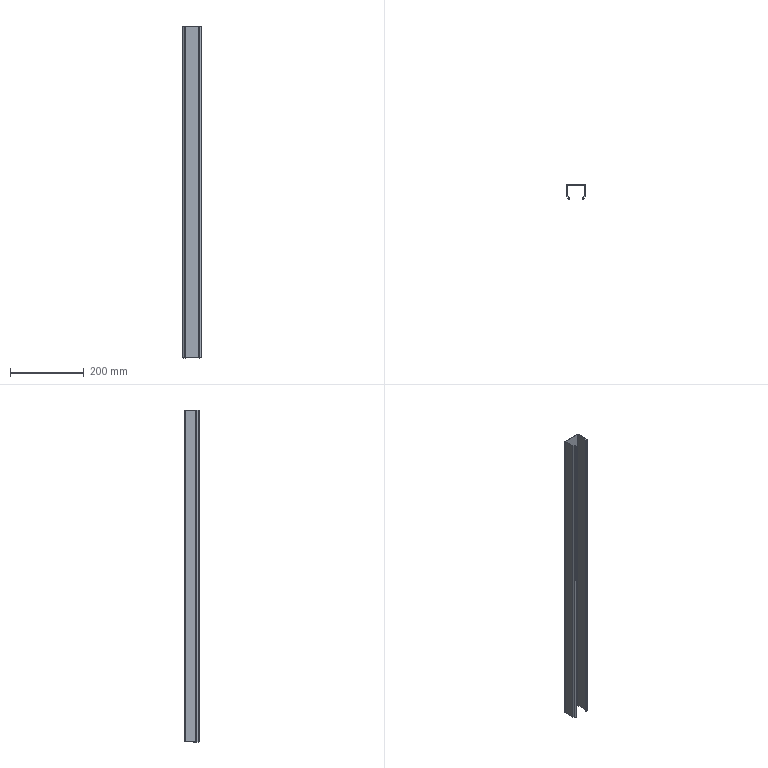Part | STEP file | 31E-01000CC13 | 1 solid | 28 faces | box 50 x 38.192 x 900 mm | volume 148176 mm3 | plane 16 | cylinder 12 | commonest cylinder face diameters 1 x4 2 x4 4 x2 26 x2
STEP:
#1=CARTESIAN_POINT('',(27.993,8.298,900.));
#2=VERTEX_POINT('',#1);
#3=CARTESIAN_POINT('',(32.281,3.187,900.));
#4=VERTEX_POINT('',#3);
#5=CARTESIAN_POINT('',(30.137,5.743,900.));
#6=DIRECTION('',(0.6428,-0.766,0.));
#7=VECTOR('',#6,1.);
#8=LINE('',#5,#7);
#9=EDGE_CURVE('',#2,#4,#8,.T.);
#10=ORIENTED_EDGE('',*,*,#9,.F.);
#11=CARTESIAN_POINT('',(27.993,8.298,0.));
#12=VERTEX_POINT('',#11);
#13=CARTESIAN_POINT('',(27.993,8.298,450.));
#14=DIRECTION('',(0.,0.,-1.));
#15=VECTOR('',#14,1.);
#16=LINE('',#13,#15);
#17=EDGE_CURVE('',#2,#12,#16,.T.);
#18=ORIENTED_EDGE('',*,*,#17,.T.);
#19=CARTESIAN_POINT('',(32.281,3.187,0.));
#20=VERTEX_POINT('',#19);
#21=CARTESIAN_POINT('',(30.137,5.743,0.));
#22=DIRECTION('',(0.6428,-0.766,0.));
#23=VECTOR('',#22,1.);
#24=LINE('',#21,#23);
#25=EDGE_CURVE('',#12,#20,#24,.T.);
#26=ORIENTED_EDGE('',*,*,#25,.T.);
#27=CARTESIAN_POINT('',(32.281,3.187,450.));
#28=DIRECTION('',(0.,0.,-1.));
#29=VECTOR('',#28,1.);
#30=LINE('',#27,#29);
#31=EDGE_CURVE('',#4,#20,#30,.T.);
#32=ORIENTED_EDGE('',*,*,#31,.F.);
#33=EDGE_LOOP('',(#10,#18,#26,#32));
#34=FACE_OUTER_BOUND('',#33,.T.);
#35=CARTESIAN_POINT('',(27.525,8.856,900.));
#36=DIRECTION('',(0.766,0.6428,0.));
#37=DIRECTION('',(-0.6428,0.766,0.));
#38=AXIS2_PLACEMENT_3D('',#35,#36,#37);
#39=PLANE('',#38);
#40=ADVANCED_FACE('',(#34),#39,.F.);
#41=CARTESIAN_POINT('',(76.325,9.293,900.));
#42=VERTEX_POINT('',#41);
#43=CARTESIAN_POINT('',(71.299,3.304,900.));
#44=VERTEX_POINT('',#43);
#45=CARTESIAN_POINT('',(73.812,6.298,900.));
#46=DIRECTION('',(-0.6428,-0.766,0.));
#47=VECTOR('',#46,1.);
#48=LINE('',#45,#47);
#49=EDGE_CURVE('',#42,#44,#48,.T.);
#50=ORIENTED_EDGE('',*,*,#49,.T.);
#51=CARTESIAN_POINT('',(71.182,2.983,900.));
#52=VERTEX_POINT('',#51);
#53=CARTESIAN_POINT('',(71.682,2.983,900.));
#54=DIRECTION('',(0.,0.,1.));
#55=AXIS2_PLACEMENT_3D('',#53,#54,$);
#56=CIRCLE('',#55,0.5);
#57=EDGE_CURVE('',#44,#52,#56,.T.);
#58=ORIENTED_EDGE('',*,*,#57,.T.);
#59=CARTESIAN_POINT('',(71.182,1.665,900.));
#60=VERTEX_POINT('',#59);
#61=CARTESIAN_POINT('',(71.182,2.324,900.));
#62=DIRECTION('',(0.,-1.,0.));
#63=VECTOR('',#62,1.);
#64=LINE('',#61,#63);
#65=EDGE_CURVE('',#52,#60,#64,.T.);
#66=ORIENTED_EDGE('',*,*,#65,.T.);
#67=CARTESIAN_POINT('',(72.397,0.6877,900.));
#68=VERTEX_POINT('',#67);
#69=CARTESIAN_POINT('',(72.182,1.665,900.));
#70=DIRECTION('',(0.,0.,1.));
#71=AXIS2_PLACEMENT_3D('',#69,#70,$);
#72=CIRCLE('',#71,1.);
#73=EDGE_CURVE('',#60,#68,#72,.T.);
#74=ORIENTED_EDGE('',*,*,#73,.T.);
#75=CARTESIAN_POINT('',(76.707,2.493,900.));
#76=VERTEX_POINT('',#75);
#77=CARTESIAN_POINT('',(69.613,13.386,900.));
#78=DIRECTION('',(0.,0.,1.));
#79=AXIS2_PLACEMENT_3D('',#77,#78,$);
#80=CIRCLE('',#79,13.);
#81=EDGE_CURVE('',#68,#76,#80,.T.);
#82=ORIENTED_EDGE('',*,*,#81,.T.);
#83=CARTESIAN_POINT('',(72.768,3.187,900.));
#84=VERTEX_POINT('',#83);
#85=CARTESIAN_POINT('',(74.738,2.84,900.));
#86=DIRECTION('',(-0.9848,0.1736,0.));
#87=VECTOR('',#86,1.);
#88=LINE('',#85,#87);
#89=EDGE_CURVE('',#76,#84,#88,.T.);
#90=ORIENTED_EDGE('',*,*,#89,.T.);
#91=CARTESIAN_POINT('',(77.057,8.298,900.));
#92=VERTEX_POINT('',#91);
#93=CARTESIAN_POINT('',(74.912,5.743,900.));
#94=DIRECTION('',(0.6428,0.766,0.));
#95=VECTOR('',#94,1.);
#96=LINE('',#93,#95);
#97=EDGE_CURVE('',#84,#92,#96,.T.);
#98=ORIENTED_EDGE('',*,*,#97,.T.);
#99=CARTESIAN_POINT('',(77.525,9.584,900.));
#100=VERTEX_POINT('',#99);
#101=CARTESIAN_POINT('',(75.525,9.584,900.));
#102=DIRECTION('',(0.,0.,1.));
#103=AXIS2_PLACEMENT_3D('',#101,#102,$);
#104=CIRCLE('',#103,2.);
#105=EDGE_CURVE('',#92,#100,#104,.T.);
#106=ORIENTED_EDGE('',*,*,#105,.T.);
#107=CARTESIAN_POINT('',(77.525,37.856,900.));
#108=VERTEX_POINT('',#107);
#109=CARTESIAN_POINT('',(77.525,23.72,900.));
#110=DIRECTION('',(0.,1.,0.));
#111=VECTOR('',#110,1.);
#112=LINE('',#109,#111);
#113=EDGE_CURVE('',#100,#108,#112,.T.);
#114=ORIENTED_EDGE('',*,*,#113,.T.);
#115=CARTESIAN_POINT('',(76.525,38.856,900.));
#116=VERTEX_POINT('',#115);
#117=CARTESIAN_POINT('',(76.525,37.856,900.));
#118=DIRECTION('',(0.,0.,1.));
#119=AXIS2_PLACEMENT_3D('',#117,#118,$);
#120=CIRCLE('',#119,1.);
#121=EDGE_CURVE('',#108,#116,#120,.T.);
#122=ORIENTED_EDGE('',*,*,#121,.T.);
#123=CARTESIAN_POINT('',(28.525,38.856,900.));
#124=VERTEX_POINT('',#123);
#125=CARTESIAN_POINT('',(52.525,38.856,900.));
#126=DIRECTION('',(-1.,0.,0.));
#127=VECTOR('',#126,1.);
#128=LINE('',#125,#127);
#129=EDGE_CURVE('',#116,#124,#128,.T.);
#130=ORIENTED_EDGE('',*,*,#129,.T.);
#131=CARTESIAN_POINT('',(27.525,37.856,900.));
#132=VERTEX_POINT('',#131);
#133=CARTESIAN_POINT('',(28.525,37.856,900.));
#134=DIRECTION('',(0.,0.,1.));
#135=AXIS2_PLACEMENT_3D('',#133,#134,$);
#136=CIRCLE('',#135,1.);
#137=EDGE_CURVE('',#124,#132,#136,.T.);
#138=ORIENTED_EDGE('',*,*,#137,.T.);
#139=CARTESIAN_POINT('',(27.525,9.584,900.));
#140=VERTEX_POINT('',#139);
#141=CARTESIAN_POINT('',(27.525,23.72,900.));
#142=DIRECTION('',(0.,-1.,0.));
#143=VECTOR('',#142,1.);
#144=LINE('',#141,#143);
#145=EDGE_CURVE('',#132,#140,#144,.T.);
#146=ORIENTED_EDGE('',*,*,#145,.T.);
#147=CARTESIAN_POINT('',(29.525,9.584,900.));
#148=DIRECTION('',(0.,0.,1.));
#149=AXIS2_PLACEMENT_3D('',#147,#148,$);
#150=CIRCLE('',#149,2.);
#151=EDGE_CURVE('',#140,#2,#150,.T.);
#152=ORIENTED_EDGE('',*,*,#151,.T.);
#153=ORIENTED_EDGE('',*,*,#9,.T.);
#154=CARTESIAN_POINT('',(28.342,2.493,900.));
#155=VERTEX_POINT('',#154);
#156=CARTESIAN_POINT('',(30.312,2.84,900.));
#157=DIRECTION('',(-0.9848,-0.1736,0.));
#158=VECTOR('',#157,1.);
#159=LINE('',#156,#158);
#160=EDGE_CURVE('',#4,#155,#159,.T.);
#161=ORIENTED_EDGE('',*,*,#160,.T.);
#162=CARTESIAN_POINT('',(32.653,0.6877,900.));
#163=VERTEX_POINT('',#162);
#164=CARTESIAN_POINT('',(35.437,13.386,900.));
#165=DIRECTION('',(0.,0.,1.));
#166=AXIS2_PLACEMENT_3D('',#164,#165,$);
#167=CIRCLE('',#166,13.);
#168=EDGE_CURVE('',#155,#163,#167,.T.);
#169=ORIENTED_EDGE('',*,*,#168,.T.);
#170=CARTESIAN_POINT('',(33.867,1.665,900.));
#171=VERTEX_POINT('',#170);
#172=CARTESIAN_POINT('',(32.867,1.665,900.));
#173=DIRECTION('',(0.,0.,1.));
#174=AXIS2_PLACEMENT_3D('',#172,#173,$);
#175=CIRCLE('',#174,1.);
#176=EDGE_CURVE('',#163,#171,#175,.T.);
#177=ORIENTED_EDGE('',*,*,#176,.T.);
#178=CARTESIAN_POINT('',(33.867,2.983,900.));
#179=VERTEX_POINT('',#178);
#180=CARTESIAN_POINT('',(33.867,2.324,900.));
#181=DIRECTION('',(0.,1.,0.));
#182=VECTOR('',#181,1.);
#183=LINE('',#180,#182);
#184=EDGE_CURVE('',#171,#179,#183,.T.);
#185=ORIENTED_EDGE('',*,*,#184,.T.);
#186=CARTESIAN_POINT('',(33.75,3.304,900.));
#187=VERTEX_POINT('',#186);
#188=CARTESIAN_POINT('',(33.367,2.983,900.));
#189=DIRECTION('',(0.,0.,1.));
#190=AXIS2_PLACEMENT_3D('',#188,#189,$);
#191=CIRCLE('',#190,0.5);
#192=EDGE_CURVE('',#179,#187,#191,.T.);
#193=ORIENTED_EDGE('',*,*,#192,.T.);
#194=CARTESIAN_POINT('',(28.725,9.293,900.));
#195=VERTEX_POINT('',#194);
#196=CARTESIAN_POINT('',(31.237,6.298,900.));
#197=DIRECTION('',(-0.6428,0.766,0.));
#198=VECTOR('',#197,1.);
#199=LINE('',#196,#198);
#200=EDGE_CURVE('',#187,#195,#199,.T.);
#201=ORIENTED_EDGE('',*,*,#200,.T.);
#202=CARTESIAN_POINT('',(28.725,37.156,900.));
#203=VERTEX_POINT('',#202);
#204=CARTESIAN_POINT('',(28.725,23.225,900.));
#205=DIRECTION('',(0.,1.,0.));
#206=VECTOR('',#205,1.);
#207=LINE('',#204,#206);
#208=EDGE_CURVE('',#195,#203,#207,.T.);
#209=ORIENTED_EDGE('',*,*,#208,.T.);
#210=CARTESIAN_POINT('',(29.225,37.656,900.));
#211=VERTEX_POINT('',#210);
#212=CARTESIAN_POINT('',(28.725,37.156,900.));
#213=CARTESIAN_POINT('',(28.725,37.219,900.));
#214=CARTESIAN_POINT('',(28.735,37.282,900.));
#215=CARTESIAN_POINT('',(28.754,37.343,900.));
#216=CARTESIAN_POINT('',(28.812,37.456,900.));
#217=CARTESIAN_POINT('',(28.902,37.546,900.));
#218=CARTESIAN_POINT('',(28.954,37.583,900.));
#219=CARTESIAN_POINT('',(29.039,37.627,900.));
#220=CARTESIAN_POINT('',(29.131,37.649,900.));
#221=CARTESIAN_POINT('',(29.162,37.654,900.));
#222=CARTESIAN_POINT('',(29.193,37.656,900.));
#223=CARTESIAN_POINT('',(29.225,37.656,900.));
#224=B_SPLINE_CURVE_WITH_KNOTS('',5,(#212,#213,#214,#215,#216,#217,#218,#219,#220,#221,#222,#223),.UNSPECIFIED.,.F.,.U.,(6,3,3,6),(0.,0.4443,0.8886,1.11),.UNSPECIFIED.);
#225=EDGE_CURVE('',#203,#211,#224,.T.);
#226=ORIENTED_EDGE('',*,*,#225,.T.);
#227=CARTESIAN_POINT('',(75.825,37.656,900.));
#228=VERTEX_POINT('',#227);
#229=CARTESIAN_POINT('',(52.525,37.656,900.));
#230=DIRECTION('',(1.,0.,0.));
#231=VECTOR('',#230,1.);
#232=LINE('',#229,#231);
#233=EDGE_CURVE('',#211,#228,#232,.T.);
#234=ORIENTED_EDGE('',*,*,#233,.T.);
#235=CARTESIAN_POINT('',(76.325,37.156,900.));
#236=VERTEX_POINT('',#235);
#237=CARTESIAN_POINT('',(75.825,37.656,900.));
#238=CARTESIAN_POINT('',(75.888,37.656,900.));
#239=CARTESIAN_POINT('',(75.95,37.646,900.));
#240=CARTESIAN_POINT('',(76.011,37.627,900.));
#241=CARTESIAN_POINT('',(76.124,37.569,900.));
#242=CARTESIAN_POINT('',(76.214,37.479,900.));
#243=CARTESIAN_POINT('',(76.252,37.427,900.));
#244=CARTESIAN_POINT('',(76.295,37.342,900.));
#245=CARTESIAN_POINT('',(76.317,37.25,900.));
#246=CARTESIAN_POINT('',(76.322,37.219,900.));
#247=CARTESIAN_POINT('',(76.325,37.187,900.));
#248=CARTESIAN_POINT('',(76.325,37.156,900.));
#249=B_SPLINE_CURVE_WITH_KNOTS('',5,(#237,#238,#239,#240,#241,#242,#243,#244,#245,#246,#247,#248),.UNSPECIFIED.,.F.,.U.,(6,3,3,6),(0.,0.4443,0.8886,1.11),.UNSPECIFIED.);
#250=EDGE_CURVE('',#228,#236,#249,.T.);
#251=ORIENTED_EDGE('',*,*,#250,.T.);
#252=CARTESIAN_POINT('',(76.325,23.225,900.));
#253=DIRECTION('',(0.,-1.,0.));
#254=VECTOR('',#253,1.);
#255=LINE('',#252,#254);
#256=EDGE_CURVE('',#236,#42,#255,.T.);
#257=ORIENTED_EDGE('',*,*,#256,.T.);
#258=EDGE_LOOP('',(#50,#58,#66,#74,#82,#90,#98,#106,#114,#122,#130,#138,#146,#152,#153,#161,#169,#177,#185,#193,#201,#209,#226,#234,#251,#257));
#259=FACE_OUTER_BOUND('',#258,.T.);
#260=CARTESIAN_POINT('',(35.437,13.386,900.));
#261=DIRECTION('',(0.,0.,1.));
#262=DIRECTION('',(1.,0.,0.));
#263=AXIS2_PLACEMENT_3D('',#260,#261,#262);
#264=PLANE('',#263);
#265=ADVANCED_FACE('',(#259),#264,.T.);
#266=ORIENTED_EDGE('',*,*,#151,.F.);
#267=CARTESIAN_POINT('',(27.525,9.584,0.));
#268=VERTEX_POINT('',#267);
#269=CARTESIAN_POINT('',(27.525,9.584,900.));
#270=DIRECTION('',(0.,0.,-1.));
#271=VECTOR('',#270,1.);
#272=LINE('',#269,#271);
#273=EDGE_CURVE('',#268,#140,#272,.F.);
#274=ORIENTED_EDGE('',*,*,#273,.F.);
#275=CARTESIAN_POINT('',(29.525,9.584,0.));
#276=DIRECTION('',(0.,0.,-1.));
#277=AXIS2_PLACEMENT_3D('',#275,#276,$);
#278=CIRCLE('',#277,2.);
#279=EDGE_CURVE('',#12,#268,#278,.T.);
#280=ORIENTED_EDGE('',*,*,#279,.F.);
#281=ORIENTED_EDGE('',*,*,#17,.F.);
#282=EDGE_LOOP('',(#266,#274,#280,#281));
#283=FACE_OUTER_BOUND('',#282,.T.);
#284=CARTESIAN_POINT('',(29.525,9.584,900.));
#285=DIRECTION('',(0.,0.,-1.));
#286=DIRECTION('',(1.,0.,0.));
#287=AXIS2_PLACEMENT_3D('',#284,#285,#286);
#288=CYLINDRICAL_SURFACE('',#287,2.);
#289=ADVANCED_FACE('',(#283),#288,.T.);
#290=CARTESIAN_POINT('',(71.182,2.983,0.));
#291=VERTEX_POINT('',#290);
#292=CARTESIAN_POINT('',(71.182,1.665,0.));
#293=VERTEX_POINT('',#292);
#294=CARTESIAN_POINT('',(71.182,2.324,0.));
#295=DIRECTION('',(0.,-1.,0.));
#296=VECTOR('',#295,1.);
#297=LINE('',#294,#296);
#298=EDGE_CURVE('',#291,#293,#297,.T.);
#299=ORIENTED_EDGE('',*,*,#298,.F.);
#300=CARTESIAN_POINT('',(71.299,3.304,0.));
#301=VERTEX_POINT('',#300);
#302=CARTESIAN_POINT('',(71.182,2.983,0.));
#303=CARTESIAN_POINT('',(71.182,3.038,0.));
#304=CARTESIAN_POINT('',(71.19,3.094,0.));
#305=CARTESIAN_POINT('',(71.206,3.149,0.));
#306=CARTESIAN_POINT('',(71.235,3.213,0.));
#307=CARTESIAN_POINT('',(71.274,3.271,0.));
#308=CARTESIAN_POINT('',(71.282,3.282,0.));
#309=CARTESIAN_POINT('',(71.29,3.293,0.));
#310=CARTESIAN_POINT('',(71.299,3.304,0.));
#311=B_SPLINE_CURVE_WITH_KNOTS('',5,(#302,#303,#304,#305,#306,#307,#308,#309,#310),.UNSPECIFIED.,.F.,.U.,(6,3,6),(0.,0.3949,0.4936),.UNSPECIFIED.);
#312=EDGE_CURVE('',#291,#301,#311,.T.);
#313=ORIENTED_EDGE('',*,*,#312,.T.);
#314=CARTESIAN_POINT('',(76.325,9.293,0.));
#315=VERTEX_POINT('',#314);
#316=CARTESIAN_POINT('',(73.812,6.298,0.));
#317=DIRECTION('',(-0.6428,-0.766,0.));
#318=VECTOR('',#317,1.);
#319=LINE('',#316,#318);
#320=EDGE_CURVE('',#315,#301,#319,.T.);
#321=ORIENTED_EDGE('',*,*,#320,.F.);
#322=CARTESIAN_POINT('',(76.325,37.156,0.));
#323=VERTEX_POINT('',#322);
#324=CARTESIAN_POINT('',(76.325,23.225,0.));
#325=DIRECTION('',(0.,-1.,0.));
#326=VECTOR('',#325,1.);
#327=LINE('',#324,#326);
#328=EDGE_CURVE('',#323,#315,#327,.T.);
#329=ORIENTED_EDGE('',*,*,#328,.F.);
#330=CARTESIAN_POINT('',(75.825,37.656,0.));
#331=VERTEX_POINT('',#330);
#332=CARTESIAN_POINT('',(75.825,37.156,0.));
#333=DIRECTION('',(0.,0.,1.));
#334=AXIS2_PLACEMENT_3D('',#332,#333,$);
#335=CIRCLE('',#334,0.5);
#336=EDGE_CURVE('',#323,#331,#335,.T.);
#337=ORIENTED_EDGE('',*,*,#336,.T.);
#338=CARTESIAN_POINT('',(29.225,37.656,0.));
#339=VERTEX_POINT('',#338);
#340=CARTESIAN_POINT('',(52.525,37.656,0.));
#341=DIRECTION('',(1.,0.,0.));
#342=VECTOR('',#341,1.);
#343=LINE('',#340,#342);
#344=EDGE_CURVE('',#339,#331,#343,.T.);
#345=ORIENTED_EDGE('',*,*,#344,.F.);
#346=CARTESIAN_POINT('',(28.725,37.156,0.));
#347=VERTEX_POINT('',#346);
#348=CARTESIAN_POINT('',(29.225,37.156,0.));
#349=DIRECTION('',(0.,0.,1.));
#350=AXIS2_PLACEMENT_3D('',#348,#349,$);
#351=CIRCLE('',#350,0.5);
#352=EDGE_CURVE('',#339,#347,#351,.T.);
#353=ORIENTED_EDGE('',*,*,#352,.T.);
#354=CARTESIAN_POINT('',(28.725,9.293,0.));
#355=VERTEX_POINT('',#354);
#356=CARTESIAN_POINT('',(28.725,23.225,0.));
#357=DIRECTION('',(0.,1.,0.));
#358=VECTOR('',#357,1.);
#359=LINE('',#356,#358);
#360=EDGE_CURVE('',#355,#347,#359,.T.);
#361=ORIENTED_EDGE('',*,*,#360,.F.);
#362=CARTESIAN_POINT('',(33.75,3.304,0.));
#363=VERTEX_POINT('',#362);
#364=CARTESIAN_POINT('',(31.237,6.298,0.));
#365=DIRECTION('',(-0.6428,0.766,0.));
#366=VECTOR('',#365,1.);
#367=LINE('',#364,#366);
#368=EDGE_CURVE('',#363,#355,#367,.T.);
#369=ORIENTED_EDGE('',*,*,#368,.F.);
#370=CARTESIAN_POINT('',(33.867,2.983,0.));
#371=VERTEX_POINT('',#370);
#372=CARTESIAN_POINT('',(33.75,3.304,0.));
#373=CARTESIAN_POINT('',(33.786,3.261,0.));
#374=CARTESIAN_POINT('',(33.816,3.213,0.));
#375=CARTESIAN_POINT('',(33.839,3.162,0.));
#376=CARTESIAN_POINT('',(33.858,3.094,0.));
#377=CARTESIAN_POINT('',(33.866,3.024,0.));
#378=CARTESIAN_POINT('',(33.867,3.01,0.));
#379=CARTESIAN_POINT('',(33.867,2.997,0.));
#380=CARTESIAN_POINT('',(33.867,2.983,0.));
#381=B_SPLINE_CURVE_WITH_KNOTS('',5,(#372,#373,#374,#375,#376,#377,#378,#379,#380),.UNSPECIFIED.,.F.,.U.,(6,3,6),(0.,0.3949,0.4936),.UNSPECIFIED.);
#382=EDGE_CURVE('',#363,#371,#381,.T.);
#383=ORIENTED_EDGE('',*,*,#382,.T.);
#384=CARTESIAN_POINT('',(33.867,1.665,0.));
#385=VERTEX_POINT('',#384);
#386=CARTESIAN_POINT('',(33.867,2.324,0.));
#387=DIRECTION('',(0.,1.,0.));
#388=VECTOR('',#387,1.);
#389=LINE('',#386,#388);
#390=EDGE_CURVE('',#385,#371,#389,.T.);
#391=ORIENTED_EDGE('',*,*,#390,.F.);
#392=CARTESIAN_POINT('',(32.653,0.6877,0.));
#393=VERTEX_POINT('',#392);
#394=CARTESIAN_POINT('',(32.867,1.665,0.));
#395=DIRECTION('',(0.,0.,1.));
#396=AXIS2_PLACEMENT_3D('',#394,#395,$);
#397=CIRCLE('',#396,1.);
#398=EDGE_CURVE('',#393,#385,#397,.T.);
#399=ORIENTED_EDGE('',*,*,#398,.F.);
#400=CARTESIAN_POINT('',(28.342,2.493,0.));
#401=VERTEX_POINT('',#400);
#402=CARTESIAN_POINT('',(35.437,13.386,0.));
#403=DIRECTION('',(0.,0.,1.));
#404=AXIS2_PLACEMENT_3D('',#402,#403,$);
#405=CIRCLE('',#404,13.);
#406=EDGE_CURVE('',#401,#393,#405,.T.);
#407=ORIENTED_EDGE('',*,*,#406,.F.);
#408=CARTESIAN_POINT('',(30.312,2.84,0.));
#409=DIRECTION('',(-0.9848,-0.1736,0.));
#410=VECTOR('',#409,1.);
#411=LINE('',#408,#410);
#412=EDGE_CURVE('',#20,#401,#411,.T.);
#413=ORIENTED_EDGE('',*,*,#412,.F.);
#414=ORIENTED_EDGE('',*,*,#25,.F.);
#415=ORIENTED_EDGE('',*,*,#279,.T.);
#416=CARTESIAN_POINT('',(27.525,37.856,0.));
#417=VERTEX_POINT('',#416);
#418=CARTESIAN_POINT('',(27.525,23.72,0.));
#419=DIRECTION('',(0.,-1.,0.));
#420=VECTOR('',#419,1.);
#421=LINE('',#418,#420);
#422=EDGE_CURVE('',#417,#268,#421,.T.);
#423=ORIENTED_EDGE('',*,*,#422,.F.);
#424=CARTESIAN_POINT('',(28.525,38.856,0.));
#425=VERTEX_POINT('',#424);
#426=CARTESIAN_POINT('',(27.525,37.856,0.));
#427=CARTESIAN_POINT('',(27.525,37.954,0.));
#428=CARTESIAN_POINT('',(27.537,38.052,0.));
#429=CARTESIAN_POINT('',(27.561,38.148,0.));
#430=CARTESIAN_POINT('',(27.632,38.332,0.));
#431=CARTESIAN_POINT('',(27.745,38.494,0.));
#432=CARTESIAN_POINT('',(27.812,38.567,0.));
#433=CARTESIAN_POINT('',(27.961,38.696,0.));
#434=CARTESIAN_POINT('',(28.137,38.786,0.));
#435=CARTESIAN_POINT('',(28.23,38.819,0.));
#436=CARTESIAN_POINT('',(28.346,38.846,0.));
#437=CARTESIAN_POINT('',(28.464,38.855,0.));
#438=CARTESIAN_POINT('',(28.484,38.856,0.));
#439=CARTESIAN_POINT('',(28.505,38.856,0.));
#440=CARTESIAN_POINT('',(28.525,38.856,0.));
#441=B_SPLINE_CURVE_WITH_KNOTS('',5,(#426,#427,#428,#429,#430,#431,#432,#433,#434,#435,#436,#437,#438,#439,#440),.UNSPECIFIED.,.F.,.U.,(6,3,3,3,6),(0.,0.6928,1.386,2.078,2.221),.UNSPECIFIED.);
#442=EDGE_CURVE('',#417,#425,#441,.T.);
#443=ORIENTED_EDGE('',*,*,#442,.T.);
#444=CARTESIAN_POINT('',(76.525,38.856,0.));
#445=VERTEX_POINT('',#444);
#446=CARTESIAN_POINT('',(52.525,38.856,0.));
#447=DIRECTION('',(-1.,0.,0.));
#448=VECTOR('',#447,1.);
#449=LINE('',#446,#448);
#450=EDGE_CURVE('',#445,#425,#449,.T.);
#451=ORIENTED_EDGE('',*,*,#450,.F.);
#452=CARTESIAN_POINT('',(77.525,37.856,0.));
#453=VERTEX_POINT('',#452);
#454=CARTESIAN_POINT('',(76.525,38.856,0.));
#455=CARTESIAN_POINT('',(76.623,38.856,0.));
#456=CARTESIAN_POINT('',(76.721,38.844,0.));
#457=CARTESIAN_POINT('',(76.817,38.82,0.));
#458=CARTESIAN_POINT('',(77.001,38.749,0.));
#459=CARTESIAN_POINT('',(77.163,38.636,0.));
#460=CARTESIAN_POINT('',(77.236,38.569,0.));
#461=CARTESIAN_POINT('',(77.365,38.42,0.));
#462=CARTESIAN_POINT('',(77.454,38.244,0.));
#463=CARTESIAN_POINT('',(77.488,38.151,0.));
#464=CARTESIAN_POINT('',(77.514,38.035,0.));
#465=CARTESIAN_POINT('',(77.523,37.917,0.));
#466=CARTESIAN_POINT('',(77.524,37.897,0.));
#467=CARTESIAN_POINT('',(77.525,37.876,0.));
#468=CARTESIAN_POINT('',(77.525,37.856,0.));
#469=B_SPLINE_CURVE_WITH_KNOTS('',5,(#454,#455,#456,#457,#458,#459,#460,#461,#462,#463,#464,#465,#466,#467,#468),.UNSPECIFIED.,.F.,.U.,(6,3,3,3,6),(0.,0.6928,1.386,2.078,2.221),.UNSPECIFIED.);
#470=EDGE_CURVE('',#445,#453,#469,.T.);
#471=ORIENTED_EDGE('',*,*,#470,.T.);
#472=CARTESIAN_POINT('',(77.525,9.584,0.));
#473=VERTEX_POINT('',#472);
#474=CARTESIAN_POINT('',(77.525,23.72,0.));
#475=DIRECTION('',(0.,1.,0.));
#476=VECTOR('',#475,1.);
#477=LINE('',#474,#476);
#478=EDGE_CURVE('',#473,#453,#477,.T.);
#479=ORIENTED_EDGE('',*,*,#478,.F.);
#480=CARTESIAN_POINT('',(77.057,8.298,0.));
#481=VERTEX_POINT('',#480);
#482=CARTESIAN_POINT('',(77.525,9.584,0.));
#483=CARTESIAN_POINT('',(77.525,9.361,0.));
#484=CARTESIAN_POINT('',(77.494,9.137,0.));
#485=CARTESIAN_POINT('',(77.431,8.92,0.));
#486=CARTESIAN_POINT('',(77.316,8.662,0.));
#487=CARTESIAN_POINT('',(77.16,8.431,0.));
#488=CARTESIAN_POINT('',(77.127,8.385,0.));
#489=CARTESIAN_POINT('',(77.093,8.341,0.));
#490=CARTESIAN_POINT('',(77.057,8.298,0.));
#491=B_SPLINE_CURVE_WITH_KNOTS('',5,(#482,#483,#484,#485,#486,#487,#488,#489,#490),.UNSPECIFIED.,.F.,.U.,(6,3,6),(0.,1.58,1.974),.UNSPECIFIED.);
#492=EDGE_CURVE('',#473,#481,#491,.T.);
#493=ORIENTED_EDGE('',*,*,#492,.T.);
#494=CARTESIAN_POINT('',(72.768,3.187,0.));
#495=VERTEX_POINT('',#494);
#496=CARTESIAN_POINT('',(74.912,5.743,0.));
#497=DIRECTION('',(0.6428,0.766,0.));
#498=VECTOR('',#497,1.);
#499=LINE('',#496,#498);
#500=EDGE_CURVE('',#495,#481,#499,.T.);
#501=ORIENTED_EDGE('',*,*,#500,.F.);
#502=CARTESIAN_POINT('',(76.707,2.493,0.));
#503=VERTEX_POINT('',#502);
#504=CARTESIAN_POINT('',(74.738,2.84,0.));
#505=DIRECTION('',(-0.9848,0.1736,0.));
#506=VECTOR('',#505,1.);
#507=LINE('',#504,#506);
#508=EDGE_CURVE('',#503,#495,#507,.T.);
#509=ORIENTED_EDGE('',*,*,#508,.F.);
#510=CARTESIAN_POINT('',(72.397,0.6877,0.));
#511=VERTEX_POINT('',#510);
#512=CARTESIAN_POINT('',(69.613,13.386,0.));
#513=DIRECTION('',(0.,0.,1.));
#514=AXIS2_PLACEMENT_3D('',#512,#513,$);
#515=CIRCLE('',#514,13.);
#516=EDGE_CURVE('',#511,#503,#515,.T.);
#517=ORIENTED_EDGE('',*,*,#516,.F.);
#518=CARTESIAN_POINT('',(72.182,1.665,0.));
#519=DIRECTION('',(0.,0.,1.));
#520=AXIS2_PLACEMENT_3D('',#518,#519,$);
#521=CIRCLE('',#520,1.);
#522=EDGE_CURVE('',#293,#511,#521,.T.);
#523=ORIENTED_EDGE('',*,*,#522,.F.);
#524=EDGE_LOOP('',(#299,#313,#321,#329,#337,#345,#353,#361,#369,#383,#391,#399,#407,#413,#414,#415,#423,#443,#451,#471,#479,#493,#501,#509,#517,#523));
#525=FACE_OUTER_BOUND('',#524,.T.);
#526=CARTESIAN_POINT('',(35.437,13.386,0.));
#527=DIRECTION('',(0.,0.,1.));
#528=DIRECTION('',(1.,0.,0.));
#529=AXIS2_PLACEMENT_3D('',#526,#527,#528);
#530=PLANE('',#529);
#531=ADVANCED_FACE('',(#525),#530,.F.);
#532=ORIENTED_EDGE('',*,*,#412,.T.);
#533=CARTESIAN_POINT('',(28.342,2.493,450.));
#534=DIRECTION('',(0.,0.,-1.));
#535=VECTOR('',#534,1.);
#536=LINE('',#533,#535);
#537=EDGE_CURVE('',#155,#401,#536,.T.);
#538=ORIENTED_EDGE('',*,*,#537,.F.);
#539=ORIENTED_EDGE('',*,*,#160,.F.);
#540=ORIENTED_EDGE('',*,*,#31,.T.);
#541=EDGE_LOOP('',(#532,#538,#539,#540));
#542=FACE_OUTER_BOUND('',#541,.T.);
#543=CARTESIAN_POINT('',(32.281,3.187,900.));
#544=DIRECTION('',(0.1736,-0.9848,0.));
#545=DIRECTION('',(0.9848,0.1736,0.));
#546=AXIS2_PLACEMENT_3D('',#543,#544,#545);
#547=PLANE('',#546);
#548=ADVANCED_FACE('',(#542),#547,.F.);
#549=ORIENTED_EDGE('',*,*,#320,.T.);
#550=CARTESIAN_POINT('',(71.299,3.304,450.));
#551=DIRECTION('',(0.,0.,1.));
#552=VECTOR('',#551,1.);
#553=LINE('',#550,#552);
#554=EDGE_CURVE('',#301,#44,#553,.T.);
#555=ORIENTED_EDGE('',*,*,#554,.T.);
#556=ORIENTED_EDGE('',*,*,#49,.F.);
#557=CARTESIAN_POINT('',(76.325,9.293,450.));
#558=DIRECTION('',(0.,0.,-1.));
#559=VECTOR('',#558,1.);
#560=LINE('',#557,#559);
#561=EDGE_CURVE('',#42,#315,#560,.T.);
#562=ORIENTED_EDGE('',*,*,#561,.T.);
#563=EDGE_LOOP('',(#549,#555,#556,#562));
#564=FACE_OUTER_BOUND('',#563,.T.);
#565=CARTESIAN_POINT('',(76.325,9.293,900.));
#566=DIRECTION('',(0.766,-0.6428,0.));
#567=DIRECTION('',(0.6428,0.766,0.));
#568=AXIS2_PLACEMENT_3D('',#565,#566,#567);
#569=PLANE('',#568);
#570=ADVANCED_FACE('',(#564),#569,.F.);
#571=ORIENTED_EDGE('',*,*,#57,.F.);
#572=ORIENTED_EDGE('',*,*,#554,.F.);
#573=ORIENTED_EDGE('',*,*,#312,.F.);
#574=CARTESIAN_POINT('',(71.182,2.983,900.));
#575=DIRECTION('',(0.,0.,-1.));
#576=VECTOR('',#575,1.);
#577=LINE('',#574,#576);
#578=EDGE_CURVE('',#52,#291,#577,.T.);
#579=ORIENTED_EDGE('',*,*,#578,.F.);
#580=EDGE_LOOP('',(#571,#572,#573,#579));
#581=FACE_OUTER_BOUND('',#580,.T.);
#582=CARTESIAN_POINT('',(71.682,2.983,900.));
#583=DIRECTION('',(0.,0.,-1.));
#584=DIRECTION('',(-1.,0.,0.));
#585=AXIS2_PLACEMENT_3D('',#582,#583,#584);
#586=CYLINDRICAL_SURFACE('',#585,0.5);
#587=ADVANCED_FACE('',(#581),#586,.T.);
#588=ORIENTED_EDGE('',*,*,#65,.F.);
#589=ORIENTED_EDGE('',*,*,#578,.T.);
#590=ORIENTED_EDGE('',*,*,#298,.T.);
#591=CARTESIAN_POINT('',(71.182,1.665,450.));
#592=DIRECTION('',(0.,0.,-1.));
#593=VECTOR('',#592,1.);
#594=LINE('',#591,#593);
#595=EDGE_CURVE('',#60,#293,#594,.T.);
#596=ORIENTED_EDGE('',*,*,#595,.F.);
#597=EDGE_LOOP('',(#588,#589,#590,#596));
#598=FACE_OUTER_BOUND('',#597,.T.);
#599=CARTESIAN_POINT('',(71.182,1.665,900.));
#600=DIRECTION('',(1.,0.,0.));
#601=DIRECTION('',(0.,0.,-1.));
#602=AXIS2_PLACEMENT_3D('',#599,#600,#601);
#603=PLANE('',#602);
#604=ADVANCED_FACE('',(#598),#603,.F.);
#605=ORIENTED_EDGE('',*,*,#522,.T.);
#606=CARTESIAN_POINT('',(72.397,0.6877,900.));
#607=DIRECTION('',(0.,0.,-1.));
#608=VECTOR('',#607,1.);
#609=LINE('',#606,#608);
#610=EDGE_CURVE('',#68,#511,#609,.T.);
#611=ORIENTED_EDGE('',*,*,#610,.F.);
#612=ORIENTED_EDGE('',*,*,#73,.F.);
#613=ORIENTED_EDGE('',*,*,#595,.T.);
#614=EDGE_LOOP('',(#605,#611,#612,#613));
#615=FACE_OUTER_BOUND('',#614,.T.);
#616=CARTESIAN_POINT('',(72.182,1.665,900.));
#617=DIRECTION('',(0.,0.,-1.));
#618=DIRECTION('',(1.,0.,0.));
#619=AXIS2_PLACEMENT_3D('',#616,#617,#618);
#620=CYLINDRICAL_SURFACE('',#619,1.);
#621=ADVANCED_FACE('',(#615),#620,.T.);
#622=ORIENTED_EDGE('',*,*,#516,.T.);
#623=CARTESIAN_POINT('',(76.707,2.493,900.));
#624=DIRECTION('',(0.,0.,-1.));
#625=VECTOR('',#624,1.);
#626=LINE('',#623,#625);
#627=EDGE_CURVE('',#76,#503,#626,.T.);
#628=ORIENTED_EDGE('',*,*,#627,.F.);
#629=ORIENTED_EDGE('',*,*,#81,.F.);
#630=ORIENTED_EDGE('',*,*,#610,.T.);
#631=EDGE_LOOP('',(#622,#628,#629,#630));
#632=FACE_OUTER_BOUND('',#631,.T.);
#633=CARTESIAN_POINT('',(69.613,13.386,900.));
#634=DIRECTION('',(0.,0.,-1.));
#635=DIRECTION('',(1.,0.,0.));
#636=AXIS2_PLACEMENT_3D('',#633,#634,#635);
#637=CYLINDRICAL_SURFACE('',#636,13.);
#638=ADVANCED_FACE('',(#632),#637,.T.);
#639=ORIENTED_EDGE('',*,*,#508,.T.);
#640=CARTESIAN_POINT('',(72.768,3.187,450.));
#641=DIRECTION('',(0.,0.,-1.));
#642=VECTOR('',#641,1.);
#643=LINE('',#640,#642);
#644=EDGE_CURVE('',#84,#495,#643,.T.);
#645=ORIENTED_EDGE('',*,*,#644,.F.);
#646=ORIENTED_EDGE('',*,*,#89,.F.);
#647=ORIENTED_EDGE('',*,*,#627,.T.);
#648=EDGE_LOOP('',(#639,#645,#646,#647));
#649=FACE_OUTER_BOUND('',#648,.T.);
#650=CARTESIAN_POINT('',(72.768,3.187,900.));
#651=DIRECTION('',(-0.1736,-0.9848,0.));
#652=DIRECTION('',(0.9848,-0.1736,0.));
#653=AXIS2_PLACEMENT_3D('',#650,#651,#652);
#654=PLANE('',#653);
#655=ADVANCED_FACE('',(#649),#654,.F.);
#656=ORIENTED_EDGE('',*,*,#500,.T.);
#657=CARTESIAN_POINT('',(77.057,8.298,450.));
#658=DIRECTION('',(0.,0.,1.));
#659=VECTOR('',#658,1.);
#660=LINE('',#657,#659);
#661=EDGE_CURVE('',#481,#92,#660,.T.);
#662=ORIENTED_EDGE('',*,*,#661,.T.);
#663=ORIENTED_EDGE('',*,*,#97,.F.);
#664=ORIENTED_EDGE('',*,*,#644,.T.);
#665=EDGE_LOOP('',(#656,#662,#663,#664));
#666=FACE_OUTER_BOUND('',#665,.T.);
#667=CARTESIAN_POINT('',(77.525,8.856,900.));
#668=DIRECTION('',(-0.766,0.6428,0.));
#669=DIRECTION('',(-0.6428,-0.766,0.));
#670=AXIS2_PLACEMENT_3D('',#667,#668,#669);
#671=PLANE('',#670);
#672=ADVANCED_FACE('',(#666),#671,.F.);
#673=ORIENTED_EDGE('',*,*,#105,.F.);
#674=ORIENTED_EDGE('',*,*,#661,.F.);
#675=ORIENTED_EDGE('',*,*,#492,.F.);
#676=CARTESIAN_POINT('',(77.525,9.584,900.));
#677=DIRECTION('',(0.,0.,-1.));
#678=VECTOR('',#677,1.);
#679=LINE('',#676,#678);
#680=EDGE_CURVE('',#100,#473,#679,.T.);
#681=ORIENTED_EDGE('',*,*,#680,.F.);
#682=EDGE_LOOP('',(#673,#674,#675,#681));
#683=FACE_OUTER_BOUND('',#682,.T.);
#684=CARTESIAN_POINT('',(75.525,9.584,900.));
#685=DIRECTION('',(0.,0.,-1.));
#686=DIRECTION('',(1.,0.,0.));
#687=AXIS2_PLACEMENT_3D('',#684,#685,#686);
#688=CYLINDRICAL_SURFACE('',#687,2.);
#689=ADVANCED_FACE('',(#683),#688,.T.);
#690=ORIENTED_EDGE('',*,*,#478,.T.);
#691=CARTESIAN_POINT('',(77.525,37.856,450.));
#692=DIRECTION('',(0.,0.,1.));
#693=VECTOR('',#692,1.);
#694=LINE('',#691,#693);
#695=EDGE_CURVE('',#453,#108,#694,.T.);
#696=ORIENTED_EDGE('',*,*,#695,.T.);
#697=ORIENTED_EDGE('',*,*,#113,.F.);
#698=ORIENTED_EDGE('',*,*,#680,.T.);
#699=EDGE_LOOP('',(#690,#696,#697,#698));
#700=FACE_OUTER_BOUND('',#699,.T.);
#701=CARTESIAN_POINT('',(77.525,8.856,900.));
#702=DIRECTION('',(-1.,0.,0.));
#703=DIRECTION('',(0.,0.,1.));
#704=AXIS2_PLACEMENT_3D('',#701,#702,#703);
#705=PLANE('',#704);
#706=ADVANCED_FACE('',(#700),#705,.F.);
#707=ORIENTED_EDGE('',*,*,#121,.F.);
#708=ORIENTED_EDGE('',*,*,#695,.F.);
#709=ORIENTED_EDGE('',*,*,#470,.F.);
#710=CARTESIAN_POINT('',(76.525,38.856,900.));
#711=DIRECTION('',(0.,0.,-1.));
#712=VECTOR('',#711,1.);
#713=LINE('',#710,#712);
#714=EDGE_CURVE('',#116,#445,#713,.T.);
#715=ORIENTED_EDGE('',*,*,#714,.F.);
#716=EDGE_LOOP('',(#707,#708,#709,#715));
#717=FACE_OUTER_BOUND('',#716,.T.);
#718=CARTESIAN_POINT('',(76.525,37.856,900.));
#719=DIRECTION('',(0.,0.,-1.));
#720=DIRECTION('',(-1.,0.,0.));
#721=AXIS2_PLACEMENT_3D('',#718,#719,#720);
#722=CYLINDRICAL_SURFACE('',#721,1.);
#723=ADVANCED_FACE('',(#717),#722,.T.);
#724=ORIENTED_EDGE('',*,*,#129,.F.);
#725=ORIENTED_EDGE('',*,*,#714,.T.);
#726=ORIENTED_EDGE('',*,*,#450,.T.);
#727=CARTESIAN_POINT('',(28.525,38.856,450.));
#728=DIRECTION('',(0.,0.,1.));
#729=VECTOR('',#728,1.);
#730=LINE('',#727,#729);
#731=EDGE_CURVE('',#425,#124,#730,.T.);
#732=ORIENTED_EDGE('',*,*,#731,.T.);
#733=EDGE_LOOP('',(#724,#725,#726,#732));
#734=FACE_OUTER_BOUND('',#733,.T.);
#735=CARTESIAN_POINT('',(27.525,38.856,900.));
#736=DIRECTION('',(0.,-1.,0.));
#737=DIRECTION('',(1.,0.,0.));
#738=AXIS2_PLACEMENT_3D('',#735,#736,#737);
#739=PLANE('',#738);
#740=ADVANCED_FACE('',(#734),#739,.F.);
#741=ORIENTED_EDGE('',*,*,#137,.F.);
#742=ORIENTED_EDGE('',*,*,#731,.F.);
#743=ORIENTED_EDGE('',*,*,#442,.F.);
#744=CARTESIAN_POINT('',(27.525,37.856,900.));
#745=DIRECTION('',(0.,0.,-1.));
#746=VECTOR('',#745,1.);
#747=LINE('',#744,#746);
#748=EDGE_CURVE('',#132,#417,#747,.T.);
#749=ORIENTED_EDGE('',*,*,#748,.F.);
#750=EDGE_LOOP('',(#741,#742,#743,#749));
#751=FACE_OUTER_BOUND('',#750,.T.);
#752=CARTESIAN_POINT('',(28.525,37.856,900.));
#753=DIRECTION('',(0.,0.,-1.));
#754=DIRECTION('',(-1.,0.,0.));
#755=AXIS2_PLACEMENT_3D('',#752,#753,#754);
#756=CYLINDRICAL_SURFACE('',#755,1.);
#757=ADVANCED_FACE('',(#751),#756,.T.);
#758=ORIENTED_EDGE('',*,*,#145,.F.);
#759=ORIENTED_EDGE('',*,*,#748,.T.);
#760=ORIENTED_EDGE('',*,*,#422,.T.);
#761=ORIENTED_EDGE('',*,*,#273,.T.);
#762=EDGE_LOOP('',(#758,#759,#760,#761));
#763=FACE_OUTER_BOUND('',#762,.T.);
#764=CARTESIAN_POINT('',(27.525,8.856,900.));
#765=DIRECTION('',(1.,0.,0.));
#766=DIRECTION('',(0.,0.,-1.));
#767=AXIS2_PLACEMENT_3D('',#764,#765,#766);
#768=PLANE('',#767);
#769=ADVANCED_FACE('',(#763),#768,.F.);
#770=ORIENTED_EDGE('',*,*,#406,.T.);
#771=CARTESIAN_POINT('',(32.653,0.6877,900.));
#772=DIRECTION('',(0.,0.,-1.));
#773=VECTOR('',#772,1.);
#774=LINE('',#771,#773);
#775=EDGE_CURVE('',#163,#393,#774,.T.);
#776=ORIENTED_EDGE('',*,*,#775,.F.);
#777=ORIENTED_EDGE('',*,*,#168,.F.);
#778=ORIENTED_EDGE('',*,*,#537,.T.);
#779=EDGE_LOOP('',(#770,#776,#777,#778));
#780=FACE_OUTER_BOUND('',#779,.T.);
#781=CARTESIAN_POINT('',(35.437,13.386,900.));
#782=DIRECTION('',(0.,0.,-1.));
#783=DIRECTION('',(1.,0.,0.));
#784=AXIS2_PLACEMENT_3D('',#781,#782,#783);
#785=CYLINDRICAL_SURFACE('',#784,13.);
#786=ADVANCED_FACE('',(#780),#785,.T.);
#787=ORIENTED_EDGE('',*,*,#398,.T.);
#788=CARTESIAN_POINT('',(33.867,1.665,900.));
#789=DIRECTION('',(0.,0.,-1.));
#790=VECTOR('',#789,1.);
#791=LINE('',#788,#790);
#792=EDGE_CURVE('',#171,#385,#791,.T.);
#793=ORIENTED_EDGE('',*,*,#792,.F.);
#794=ORIENTED_EDGE('',*,*,#176,.F.);
#795=ORIENTED_EDGE('',*,*,#775,.T.);
#796=EDGE_LOOP('',(#787,#793,#794,#795));
#797=FACE_OUTER_BOUND('',#796,.T.);
#798=CARTESIAN_POINT('',(32.867,1.665,900.));
#799=DIRECTION('',(0.,0.,-1.));
#800=DIRECTION('',(1.,0.,0.));
#801=AXIS2_PLACEMENT_3D('',#798,#799,#800);
#802=CYLINDRICAL_SURFACE('',#801,1.);
#803=ADVANCED_FACE('',(#797),#802,.T.);
#804=ORIENTED_EDGE('',*,*,#390,.T.);
#805=CARTESIAN_POINT('',(33.867,2.983,450.));
#806=DIRECTION('',(0.,0.,1.));
#807=VECTOR('',#806,1.);
#808=LINE('',#805,#807);
#809=EDGE_CURVE('',#371,#179,#808,.T.);
#810=ORIENTED_EDGE('',*,*,#809,.T.);
#811=ORIENTED_EDGE('',*,*,#184,.F.);
#812=ORIENTED_EDGE('',*,*,#792,.T.);
#813=EDGE_LOOP('',(#804,#810,#811,#812));
#814=FACE_OUTER_BOUND('',#813,.T.);
#815=CARTESIAN_POINT('',(33.867,1.665,900.));
#816=DIRECTION('',(-1.,0.,0.));
#817=DIRECTION('',(0.,0.,1.));
#818=AXIS2_PLACEMENT_3D('',#815,#816,#817);
#819=PLANE('',#818);
#820=ADVANCED_FACE('',(#814),#819,.F.);
#821=ORIENTED_EDGE('',*,*,#192,.F.);
#822=ORIENTED_EDGE('',*,*,#809,.F.);
#823=ORIENTED_EDGE('',*,*,#382,.F.);
#824=CARTESIAN_POINT('',(33.75,3.304,900.));
#825=DIRECTION('',(0.,0.,-1.));
#826=VECTOR('',#825,1.);
#827=LINE('',#824,#826);
#828=EDGE_CURVE('',#187,#363,#827,.T.);
#829=ORIENTED_EDGE('',*,*,#828,.F.);
#830=EDGE_LOOP('',(#821,#822,#823,#829));
#831=FACE_OUTER_BOUND('',#830,.T.);
#832=CARTESIAN_POINT('',(33.367,2.983,900.));
#833=DIRECTION('',(0.,0.,-1.));
#834=DIRECTION('',(-1.,0.,0.));
#835=AXIS2_PLACEMENT_3D('',#832,#833,#834);
#836=CYLINDRICAL_SURFACE('',#835,0.5);
#837=ADVANCED_FACE('',(#831),#836,.T.);
#838=ORIENTED_EDGE('',*,*,#200,.F.);
#839=ORIENTED_EDGE('',*,*,#828,.T.);
#840=ORIENTED_EDGE('',*,*,#368,.T.);
#841=CARTESIAN_POINT('',(28.725,9.293,450.));
#842=DIRECTION('',(0.,0.,-1.));
#843=VECTOR('',#842,1.);
#844=LINE('',#841,#843);
#845=EDGE_CURVE('',#195,#355,#844,.T.);
#846=ORIENTED_EDGE('',*,*,#845,.F.);
#847=EDGE_LOOP('',(#838,#839,#840,#846));
#848=FACE_OUTER_BOUND('',#847,.T.);
#849=CARTESIAN_POINT('',(28.725,9.293,900.));
#850=DIRECTION('',(-0.766,-0.6428,0.));
#851=DIRECTION('',(0.6428,-0.766,0.));
#852=AXIS2_PLACEMENT_3D('',#849,#850,#851);
#853=PLANE('',#852);
#854=ADVANCED_FACE('',(#848),#853,.F.);
#855=ORIENTED_EDGE('',*,*,#360,.T.);
#856=CARTESIAN_POINT('',(28.725,37.156,450.));
#857=DIRECTION('',(0.,0.,1.));
#858=VECTOR('',#857,1.);
#859=LINE('',#856,#858);
#860=EDGE_CURVE('',#347,#203,#859,.T.);
#861=ORIENTED_EDGE('',*,*,#860,.T.);
#862=ORIENTED_EDGE('',*,*,#208,.F.);
#863=ORIENTED_EDGE('',*,*,#845,.T.);
#864=EDGE_LOOP('',(#855,#861,#862,#863));
#865=FACE_OUTER_BOUND('',#864,.T.);
#866=CARTESIAN_POINT('',(28.725,9.293,900.));
#867=DIRECTION('',(-1.,0.,0.));
#868=DIRECTION('',(0.,0.,1.));
#869=AXIS2_PLACEMENT_3D('',#866,#867,#868);
#870=PLANE('',#869);
#871=ADVANCED_FACE('',(#865),#870,.F.);
#872=ORIENTED_EDGE('',*,*,#225,.F.);
#873=ORIENTED_EDGE('',*,*,#860,.F.);
#874=ORIENTED_EDGE('',*,*,#352,.F.);
#875=CARTESIAN_POINT('',(29.225,37.656,900.));
#876=DIRECTION('',(0.,0.,1.));
#877=VECTOR('',#876,1.);
#878=LINE('',#875,#877);
#879=EDGE_CURVE('',#211,#339,#878,.F.);
#880=ORIENTED_EDGE('',*,*,#879,.F.);
#881=EDGE_LOOP('',(#872,#873,#874,#880));
#882=FACE_OUTER_BOUND('',#881,.T.);
#883=CARTESIAN_POINT('',(29.225,37.156,900.));
#884=DIRECTION('',(0.,0.,1.));
#885=DIRECTION('',(1.,0.,0.));
#886=AXIS2_PLACEMENT_3D('',#883,#884,#885);
#887=CYLINDRICAL_SURFACE('',#886,0.5);
#888=ADVANCED_FACE('',(#882),#887,.F.);
#889=ORIENTED_EDGE('',*,*,#344,.T.);
#890=CARTESIAN_POINT('',(75.825,37.656,450.));
#891=DIRECTION('',(0.,0.,1.));
#892=VECTOR('',#891,1.);
#893=LINE('',#890,#892);
#894=EDGE_CURVE('',#331,#228,#893,.T.);
#895=ORIENTED_EDGE('',*,*,#894,.T.);
#896=ORIENTED_EDGE('',*,*,#233,.F.);
#897=ORIENTED_EDGE('',*,*,#879,.T.);
#898=EDGE_LOOP('',(#889,#895,#896,#897));
#899=FACE_OUTER_BOUND('',#898,.T.);
#900=CARTESIAN_POINT('',(28.725,37.656,900.));
#901=DIRECTION('',(0.,1.,0.));
#902=DIRECTION('',(-1.,0.,0.));
#903=AXIS2_PLACEMENT_3D('',#900,#901,#902);
#904=PLANE('',#903);
#905=ADVANCED_FACE('',(#899),#904,.F.);
#906=ORIENTED_EDGE('',*,*,#250,.F.);
#907=ORIENTED_EDGE('',*,*,#894,.F.);
#908=ORIENTED_EDGE('',*,*,#336,.F.);
#909=CARTESIAN_POINT('',(76.325,37.156,900.));
#910=DIRECTION('',(0.,0.,1.));
#911=VECTOR('',#910,1.);
#912=LINE('',#909,#911);
#913=EDGE_CURVE('',#236,#323,#912,.F.);
#914=ORIENTED_EDGE('',*,*,#913,.F.);
#915=EDGE_LOOP('',(#906,#907,#908,#914));
#916=FACE_OUTER_BOUND('',#915,.T.);
#917=CARTESIAN_POINT('',(75.825,37.156,900.));
#918=DIRECTION('',(0.,0.,1.));
#919=DIRECTION('',(1.,0.,0.));
#920=AXIS2_PLACEMENT_3D('',#917,#918,#919);
#921=CYLINDRICAL_SURFACE('',#920,0.5);
#922=ADVANCED_FACE('',(#916),#921,.F.);
#923=ORIENTED_EDGE('',*,*,#256,.F.);
#924=ORIENTED_EDGE('',*,*,#913,.T.);
#925=ORIENTED_EDGE('',*,*,#328,.T.);
#926=ORIENTED_EDGE('',*,*,#561,.F.);
#927=EDGE_LOOP('',(#923,#924,#925,#926));
#928=FACE_OUTER_BOUND('',#927,.T.);
#929=CARTESIAN_POINT('',(76.325,9.293,900.));
#930=DIRECTION('',(1.,0.,0.));
#931=DIRECTION('',(0.,1.,0.));
#932=AXIS2_PLACEMENT_3D('',#929,#930,#931);
#933=PLANE('',#932);
#934=ADVANCED_FACE('',(#928),#933,.F.);
#935=CLOSED_SHELL('',(#40,#265,#289,#531,#548,#570,#587,#604,#621,#638,#655,#672,#689,#706,#723,#740,#757,#769,#786,#803,#820,#837,#854,#871,#888,#905,#922,#934));
#936=MANIFOLD_SOLID_BREP('',#935);
#937=(LENGTH_UNIT()NAMED_UNIT(*)SI_UNIT(.MILLI.,.METRE.));
#938=UNCERTAINTY_MEASURE_WITH_UNIT(LENGTH_MEASURE(0.005),#937,'','');
#939=(NAMED_UNIT(*)PLANE_ANGLE_UNIT()SI_UNIT($,.RADIAN.));
#940=(NAMED_UNIT(*)SI_UNIT($,.STERADIAN.)SOLID_ANGLE_UNIT());
#941=(GEOMETRIC_REPRESENTATION_CONTEXT(3)GLOBAL_UNCERTAINTY_ASSIGNED_CONTEXT((#938))GLOBAL_UNIT_ASSIGNED_CONTEXT((#937,#939,#940))REPRESENTATION_CONTEXT('',''));
#942=ADVANCED_BREP_SHAPE_REPRESENTATION('',(#936),#941);